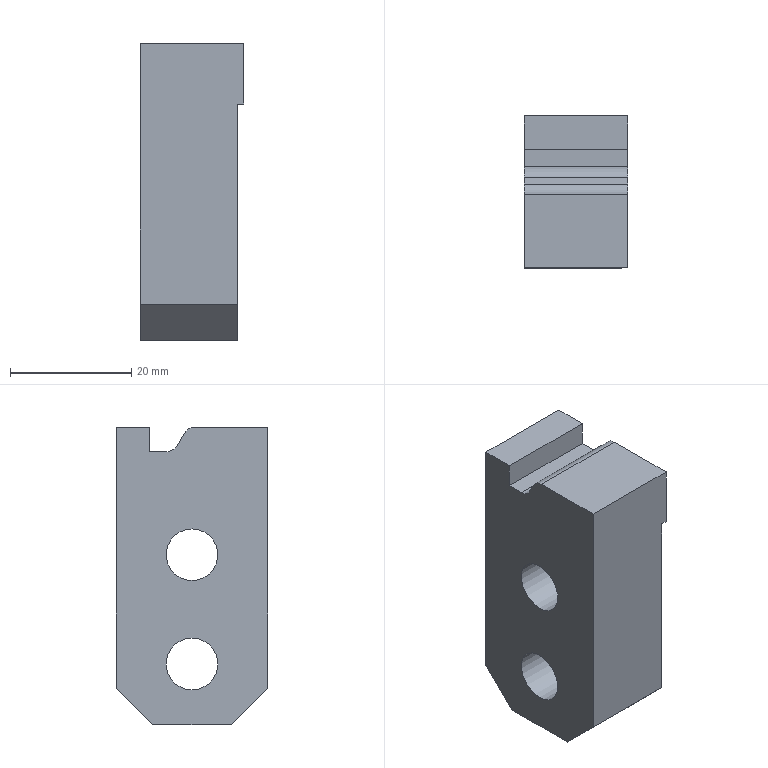Part | STEP file | gslz 2016.10.28-13_id1710_x_t | 1 solid | 22 faces | box 17 x 25 x 49 mm | volume 15358 mm3 | plane 16 | cylinder 6 | commonest cylinder face diameters 4 x2 8.5 x2 14 x2